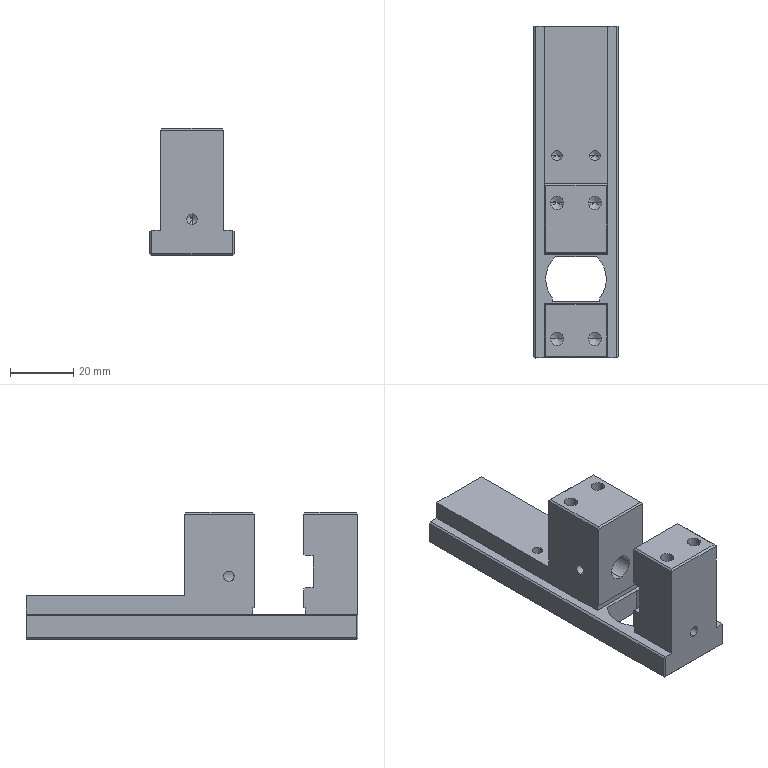Part | STEP file | displacement block | 1 solid | 84 faces | box 26.6 x 105 x 40.2 mm | volume 48167 mm3 | plane 45 | cylinder 23 | cone 16 | commonest cylinder face diameters 3.3 x8 4.2 x8 19.2 x3 6.8 x2 8 x2